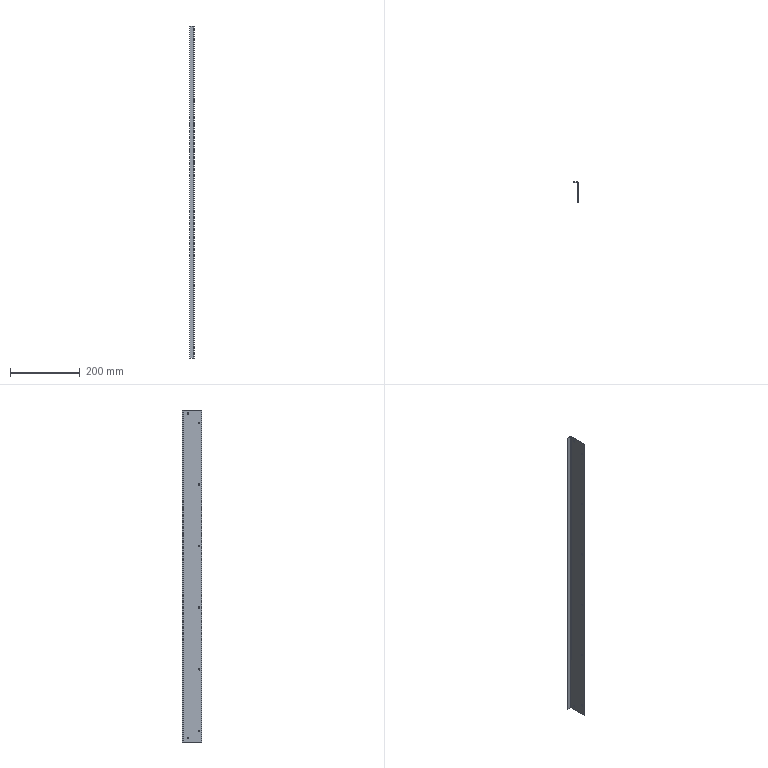Part | STEP file | 866-BDO024-95-07A_default | 1 solid | 26 faces | box 13.5 x 56.5 x 954 mm | volume 96451 mm3 | cylinder 18 | plane 8 | commonest cylinder face diameters 4.5 x16 3 x1 6 x1
STEP:
#1=CARTESIAN_POINT('',(1.5,40.,9.25));
#2=VERTEX_POINT('',#1);
#3=CARTESIAN_POINT('',(1.5,40.,13.75));
#4=VERTEX_POINT('',#3);
#5=CARTESIAN_POINT('',(1.5,40.,11.5));
#6=DIRECTION('',(-1.,0.,0.));
#7=DIRECTION('',(0.,0.,1.));
#8=AXIS2_PLACEMENT_3D('',#5,#6,#7);
#9=CIRCLE('',#8,2.25);
#10=EDGE_CURVE('',#2,#4,#9,.T.);
#11=ORIENTED_EDGE('',*,*,#10,.F.);
#12=CARTESIAN_POINT('',(0.,40.,9.25));
#13=VERTEX_POINT('',#12);
#14=CARTESIAN_POINT('',(0.,40.,9.25));
#15=DIRECTION('',(-1.,0.,0.));
#16=VECTOR('',#15,1000.);
#17=LINE('',#14,#16);
#18=EDGE_CURVE('',#2,#13,#17,.T.);
#19=ORIENTED_EDGE('',*,*,#18,.T.);
#20=CARTESIAN_POINT('',(0.,40.,13.75));
#21=VERTEX_POINT('',#20);
#22=CARTESIAN_POINT('',(0.,40.,11.5));
#23=DIRECTION('',(1.,0.,0.));
#24=DIRECTION('',(0.,0.,1.));
#25=AXIS2_PLACEMENT_3D('',#22,#23,#24);
#26=CIRCLE('',#25,2.25);
#27=EDGE_CURVE('',#21,#13,#26,.T.);
#28=ORIENTED_EDGE('',*,*,#27,.F.);
#29=CARTESIAN_POINT('',(0.,40.,13.75));
#30=DIRECTION('',(-1.,0.,0.));
#31=VECTOR('',#30,1000.);
#32=LINE('',#29,#31);
#33=EDGE_CURVE('',#4,#21,#32,.T.);
#34=ORIENTED_EDGE('',*,*,#33,.F.);
#35=EDGE_LOOP('',(#11,#19,#28,#34));
#36=FACE_OUTER_BOUND('',#35,.T.);
#37=CARTESIAN_POINT('',(0.,40.,11.5));
#38=DIRECTION('',(-1.,0.,0.));
#39=DIRECTION('',(0.,0.,1.));
#40=AXIS2_PLACEMENT_3D('',#37,#38,#39);
#41=CYLINDRICAL_SURFACE('',#40,2.25);
#42=ADVANCED_FACE('',(#36),#41,.F.);
#43=CARTESIAN_POINT('',(1.5,40.,941.75));
#44=VERTEX_POINT('',#43);
#45=CARTESIAN_POINT('',(1.5,40.,946.25));
#46=VERTEX_POINT('',#45);
#47=CARTESIAN_POINT('',(1.5,40.,944.));
#48=DIRECTION('',(-1.,0.,0.));
#49=DIRECTION('',(0.,0.,1.));
#50=AXIS2_PLACEMENT_3D('',#47,#48,#49);
#51=CIRCLE('',#50,2.25);
#52=EDGE_CURVE('',#44,#46,#51,.T.);
#53=ORIENTED_EDGE('',*,*,#52,.F.);
#54=CARTESIAN_POINT('',(0.,40.,941.75));
#55=VERTEX_POINT('',#54);
#56=CARTESIAN_POINT('',(0.,40.,941.75));
#57=DIRECTION('',(-1.,0.,0.));
#58=VECTOR('',#57,1000.);
#59=LINE('',#56,#58);
#60=EDGE_CURVE('',#44,#55,#59,.T.);
#61=ORIENTED_EDGE('',*,*,#60,.T.);
#62=CARTESIAN_POINT('',(0.,40.,946.25));
#63=VERTEX_POINT('',#62);
#64=CARTESIAN_POINT('',(0.,40.,944.));
#65=DIRECTION('',(1.,0.,0.));
#66=DIRECTION('',(0.,0.,1.));
#67=AXIS2_PLACEMENT_3D('',#64,#65,#66);
#68=CIRCLE('',#67,2.25);
#69=EDGE_CURVE('',#63,#55,#68,.T.);
#70=ORIENTED_EDGE('',*,*,#69,.F.);
#71=CARTESIAN_POINT('',(0.,40.,946.25));
#72=DIRECTION('',(-1.,0.,0.));
#73=VECTOR('',#72,1000.);
#74=LINE('',#71,#73);
#75=EDGE_CURVE('',#46,#63,#74,.T.);
#76=ORIENTED_EDGE('',*,*,#75,.F.);
#77=EDGE_LOOP('',(#53,#61,#70,#76));
#78=FACE_OUTER_BOUND('',#77,.T.);
#79=CARTESIAN_POINT('',(0.,40.,944.));
#80=DIRECTION('',(-1.,0.,0.));
#81=DIRECTION('',(0.,0.,1.));
#82=AXIS2_PLACEMENT_3D('',#79,#80,#81);
#83=CYLINDRICAL_SURFACE('',#82,2.25);
#84=ADVANCED_FACE('',(#78),#83,.F.);
#85=CARTESIAN_POINT('',(1.5,7.5,914.75));
#86=VERTEX_POINT('',#85);
#87=CARTESIAN_POINT('',(1.5,7.5,919.25));
#88=VERTEX_POINT('',#87);
#89=CARTESIAN_POINT('',(1.5,7.5,917.));
#90=DIRECTION('',(-1.,0.,0.));
#91=DIRECTION('',(0.,0.,1.));
#92=AXIS2_PLACEMENT_3D('',#89,#90,#91);
#93=CIRCLE('',#92,2.25);
#94=EDGE_CURVE('',#86,#88,#93,.T.);
#95=ORIENTED_EDGE('',*,*,#94,.F.);
#96=CARTESIAN_POINT('',(0.,7.5,914.75));
#97=VERTEX_POINT('',#96);
#98=CARTESIAN_POINT('',(0.,7.5,914.75));
#99=DIRECTION('',(-1.,0.,0.));
#100=VECTOR('',#99,1000.);
#101=LINE('',#98,#100);
#102=EDGE_CURVE('',#86,#97,#101,.T.);
#103=ORIENTED_EDGE('',*,*,#102,.T.);
#104=CARTESIAN_POINT('',(0.,7.5,919.25));
#105=VERTEX_POINT('',#104);
#106=CARTESIAN_POINT('',(0.,7.5,917.));
#107=DIRECTION('',(1.,0.,0.));
#108=DIRECTION('',(0.,0.,1.));
#109=AXIS2_PLACEMENT_3D('',#106,#107,#108);
#110=CIRCLE('',#109,2.25);
#111=EDGE_CURVE('',#105,#97,#110,.T.);
#112=ORIENTED_EDGE('',*,*,#111,.F.);
#113=CARTESIAN_POINT('',(0.,7.5,919.25));
#114=DIRECTION('',(-1.,0.,0.));
#115=VECTOR('',#114,1000.);
#116=LINE('',#113,#115);
#117=EDGE_CURVE('',#88,#105,#116,.T.);
#118=ORIENTED_EDGE('',*,*,#117,.F.);
#119=EDGE_LOOP('',(#95,#103,#112,#118));
#120=FACE_OUTER_BOUND('',#119,.T.);
#121=CARTESIAN_POINT('',(0.,7.5,917.));
#122=DIRECTION('',(-1.,0.,0.));
#123=DIRECTION('',(0.,0.,1.));
#124=AXIS2_PLACEMENT_3D('',#121,#122,#123);
#125=CYLINDRICAL_SURFACE('',#124,2.25);
#126=ADVANCED_FACE('',(#120),#125,.F.);
#127=CARTESIAN_POINT('',(1.5,7.5,737.75));
#128=VERTEX_POINT('',#127);
#129=CARTESIAN_POINT('',(1.5,7.5,742.25));
#130=VERTEX_POINT('',#129);
#131=CARTESIAN_POINT('',(1.5,7.5,740.));
#132=DIRECTION('',(-1.,0.,0.));
#133=DIRECTION('',(0.,0.,1.));
#134=AXIS2_PLACEMENT_3D('',#131,#132,#133);
#135=CIRCLE('',#134,2.25);
#136=EDGE_CURVE('',#128,#130,#135,.T.);
#137=ORIENTED_EDGE('',*,*,#136,.F.);
#138=CARTESIAN_POINT('',(0.,7.5,737.75));
#139=VERTEX_POINT('',#138);
#140=CARTESIAN_POINT('',(0.,7.5,737.75));
#141=DIRECTION('',(-1.,0.,0.));
#142=VECTOR('',#141,1000.);
#143=LINE('',#140,#142);
#144=EDGE_CURVE('',#128,#139,#143,.T.);
#145=ORIENTED_EDGE('',*,*,#144,.T.);
#146=CARTESIAN_POINT('',(0.,7.5,742.25));
#147=VERTEX_POINT('',#146);
#148=CARTESIAN_POINT('',(0.,7.5,740.));
#149=DIRECTION('',(1.,0.,0.));
#150=DIRECTION('',(0.,0.,1.));
#151=AXIS2_PLACEMENT_3D('',#148,#149,#150);
#152=CIRCLE('',#151,2.25);
#153=EDGE_CURVE('',#147,#139,#152,.T.);
#154=ORIENTED_EDGE('',*,*,#153,.F.);
#155=CARTESIAN_POINT('',(0.,7.5,742.25));
#156=DIRECTION('',(-1.,0.,0.));
#157=VECTOR('',#156,1000.);
#158=LINE('',#155,#157);
#159=EDGE_CURVE('',#130,#147,#158,.T.);
#160=ORIENTED_EDGE('',*,*,#159,.F.);
#161=EDGE_LOOP('',(#137,#145,#154,#160));
#162=FACE_OUTER_BOUND('',#161,.T.);
#163=CARTESIAN_POINT('',(0.,7.5,740.));
#164=DIRECTION('',(-1.,0.,0.));
#165=DIRECTION('',(0.,0.,1.));
#166=AXIS2_PLACEMENT_3D('',#163,#164,#165);
#167=CYLINDRICAL_SURFACE('',#166,2.25);
#168=ADVANCED_FACE('',(#162),#167,.F.);
#169=CARTESIAN_POINT('',(1.5,7.5,560.75));
#170=VERTEX_POINT('',#169);
#171=CARTESIAN_POINT('',(1.5,7.5,565.25));
#172=VERTEX_POINT('',#171);
#173=CARTESIAN_POINT('',(1.5,7.5,563.));
#174=DIRECTION('',(-1.,0.,0.));
#175=DIRECTION('',(0.,0.,1.));
#176=AXIS2_PLACEMENT_3D('',#173,#174,#175);
#177=CIRCLE('',#176,2.25);
#178=EDGE_CURVE('',#170,#172,#177,.T.);
#179=ORIENTED_EDGE('',*,*,#178,.F.);
#180=CARTESIAN_POINT('',(0.,7.5,560.75));
#181=VERTEX_POINT('',#180);
#182=CARTESIAN_POINT('',(0.,7.5,560.75));
#183=DIRECTION('',(-1.,0.,0.));
#184=VECTOR('',#183,1000.);
#185=LINE('',#182,#184);
#186=EDGE_CURVE('',#170,#181,#185,.T.);
#187=ORIENTED_EDGE('',*,*,#186,.T.);
#188=CARTESIAN_POINT('',(0.,7.5,565.25));
#189=VERTEX_POINT('',#188);
#190=CARTESIAN_POINT('',(0.,7.5,563.));
#191=DIRECTION('',(1.,0.,0.));
#192=DIRECTION('',(0.,0.,1.));
#193=AXIS2_PLACEMENT_3D('',#190,#191,#192);
#194=CIRCLE('',#193,2.25);
#195=EDGE_CURVE('',#189,#181,#194,.T.);
#196=ORIENTED_EDGE('',*,*,#195,.F.);
#197=CARTESIAN_POINT('',(0.,7.5,565.25));
#198=DIRECTION('',(-1.,0.,0.));
#199=VECTOR('',#198,1000.);
#200=LINE('',#197,#199);
#201=EDGE_CURVE('',#172,#189,#200,.T.);
#202=ORIENTED_EDGE('',*,*,#201,.F.);
#203=EDGE_LOOP('',(#179,#187,#196,#202));
#204=FACE_OUTER_BOUND('',#203,.T.);
#205=CARTESIAN_POINT('',(0.,7.5,563.));
#206=DIRECTION('',(-1.,0.,0.));
#207=DIRECTION('',(0.,0.,1.));
#208=AXIS2_PLACEMENT_3D('',#205,#206,#207);
#209=CYLINDRICAL_SURFACE('',#208,2.25);
#210=ADVANCED_FACE('',(#204),#209,.F.);
#211=CARTESIAN_POINT('',(1.5,7.5,383.75));
#212=VERTEX_POINT('',#211);
#213=CARTESIAN_POINT('',(1.5,7.5,388.25));
#214=VERTEX_POINT('',#213);
#215=CARTESIAN_POINT('',(1.5,7.5,386.));
#216=DIRECTION('',(-1.,0.,0.));
#217=DIRECTION('',(0.,0.,1.));
#218=AXIS2_PLACEMENT_3D('',#215,#216,#217);
#219=CIRCLE('',#218,2.25);
#220=EDGE_CURVE('',#212,#214,#219,.T.);
#221=ORIENTED_EDGE('',*,*,#220,.F.);
#222=CARTESIAN_POINT('',(0.,7.5,383.75));
#223=VERTEX_POINT('',#222);
#224=CARTESIAN_POINT('',(0.,7.5,383.75));
#225=DIRECTION('',(-1.,0.,0.));
#226=VECTOR('',#225,1000.);
#227=LINE('',#224,#226);
#228=EDGE_CURVE('',#212,#223,#227,.T.);
#229=ORIENTED_EDGE('',*,*,#228,.T.);
#230=CARTESIAN_POINT('',(0.,7.5,388.25));
#231=VERTEX_POINT('',#230);
#232=CARTESIAN_POINT('',(0.,7.5,386.));
#233=DIRECTION('',(1.,0.,0.));
#234=DIRECTION('',(0.,0.,1.));
#235=AXIS2_PLACEMENT_3D('',#232,#233,#234);
#236=CIRCLE('',#235,2.25);
#237=EDGE_CURVE('',#231,#223,#236,.T.);
#238=ORIENTED_EDGE('',*,*,#237,.F.);
#239=CARTESIAN_POINT('',(0.,7.5,388.25));
#240=DIRECTION('',(-1.,0.,0.));
#241=VECTOR('',#240,1000.);
#242=LINE('',#239,#241);
#243=EDGE_CURVE('',#214,#231,#242,.T.);
#244=ORIENTED_EDGE('',*,*,#243,.F.);
#245=EDGE_LOOP('',(#221,#229,#238,#244));
#246=FACE_OUTER_BOUND('',#245,.T.);
#247=CARTESIAN_POINT('',(0.,7.5,386.));
#248=DIRECTION('',(-1.,0.,0.));
#249=DIRECTION('',(0.,0.,1.));
#250=AXIS2_PLACEMENT_3D('',#247,#248,#249);
#251=CYLINDRICAL_SURFACE('',#250,2.25);
#252=ADVANCED_FACE('',(#246),#251,.F.);
#253=CARTESIAN_POINT('',(1.5,7.5,206.75));
#254=VERTEX_POINT('',#253);
#255=CARTESIAN_POINT('',(1.5,7.5,211.25));
#256=VERTEX_POINT('',#255);
#257=CARTESIAN_POINT('',(1.5,7.5,209.));
#258=DIRECTION('',(-1.,0.,0.));
#259=DIRECTION('',(0.,0.,1.));
#260=AXIS2_PLACEMENT_3D('',#257,#258,#259);
#261=CIRCLE('',#260,2.25);
#262=EDGE_CURVE('',#254,#256,#261,.T.);
#263=ORIENTED_EDGE('',*,*,#262,.F.);
#264=CARTESIAN_POINT('',(0.,7.5,206.75));
#265=VERTEX_POINT('',#264);
#266=CARTESIAN_POINT('',(0.,7.5,206.75));
#267=DIRECTION('',(-1.,0.,0.));
#268=VECTOR('',#267,1000.);
#269=LINE('',#266,#268);
#270=EDGE_CURVE('',#254,#265,#269,.T.);
#271=ORIENTED_EDGE('',*,*,#270,.T.);
#272=CARTESIAN_POINT('',(0.,7.5,211.25));
#273=VERTEX_POINT('',#272);
#274=CARTESIAN_POINT('',(0.,7.5,209.));
#275=DIRECTION('',(1.,0.,0.));
#276=DIRECTION('',(0.,0.,1.));
#277=AXIS2_PLACEMENT_3D('',#274,#275,#276);
#278=CIRCLE('',#277,2.25);
#279=EDGE_CURVE('',#273,#265,#278,.T.);
#280=ORIENTED_EDGE('',*,*,#279,.F.);
#281=CARTESIAN_POINT('',(0.,7.5,211.25));
#282=DIRECTION('',(-1.,0.,0.));
#283=VECTOR('',#282,1000.);
#284=LINE('',#281,#283);
#285=EDGE_CURVE('',#256,#273,#284,.T.);
#286=ORIENTED_EDGE('',*,*,#285,.F.);
#287=EDGE_LOOP('',(#263,#271,#280,#286));
#288=FACE_OUTER_BOUND('',#287,.T.);
#289=CARTESIAN_POINT('',(0.,7.5,209.));
#290=DIRECTION('',(-1.,0.,0.));
#291=DIRECTION('',(0.,0.,1.));
#292=AXIS2_PLACEMENT_3D('',#289,#290,#291);
#293=CYLINDRICAL_SURFACE('',#292,2.25);
#294=ADVANCED_FACE('',(#288),#293,.F.);
#295=CARTESIAN_POINT('',(1.5,7.5,29.75));
#296=VERTEX_POINT('',#295);
#297=CARTESIAN_POINT('',(1.5,7.5,34.25));
#298=VERTEX_POINT('',#297);
#299=CARTESIAN_POINT('',(1.5,7.5,32.));
#300=DIRECTION('',(-1.,0.,0.));
#301=DIRECTION('',(0.,0.,1.));
#302=AXIS2_PLACEMENT_3D('',#299,#300,#301);
#303=CIRCLE('',#302,2.25);
#304=EDGE_CURVE('',#296,#298,#303,.T.);
#305=ORIENTED_EDGE('',*,*,#304,.F.);
#306=CARTESIAN_POINT('',(0.,7.5,29.75));
#307=VERTEX_POINT('',#306);
#308=CARTESIAN_POINT('',(0.,7.5,29.75));
#309=DIRECTION('',(-1.,0.,0.));
#310=VECTOR('',#309,1000.);
#311=LINE('',#308,#310);
#312=EDGE_CURVE('',#296,#307,#311,.T.);
#313=ORIENTED_EDGE('',*,*,#312,.T.);
#314=CARTESIAN_POINT('',(0.,7.5,34.25));
#315=VERTEX_POINT('',#314);
#316=CARTESIAN_POINT('',(0.,7.5,32.));
#317=DIRECTION('',(1.,0.,0.));
#318=DIRECTION('',(0.,0.,1.));
#319=AXIS2_PLACEMENT_3D('',#316,#317,#318);
#320=CIRCLE('',#319,2.25);
#321=EDGE_CURVE('',#315,#307,#320,.T.);
#322=ORIENTED_EDGE('',*,*,#321,.F.);
#323=CARTESIAN_POINT('',(0.,7.5,34.25));
#324=DIRECTION('',(-1.,0.,0.));
#325=VECTOR('',#324,1000.);
#326=LINE('',#323,#325);
#327=EDGE_CURVE('',#298,#315,#326,.T.);
#328=ORIENTED_EDGE('',*,*,#327,.F.);
#329=EDGE_LOOP('',(#305,#313,#322,#328));
#330=FACE_OUTER_BOUND('',#329,.T.);
#331=CARTESIAN_POINT('',(0.,7.5,32.));
#332=DIRECTION('',(-1.,0.,0.));
#333=DIRECTION('',(0.,0.,1.));
#334=AXIS2_PLACEMENT_3D('',#331,#332,#333);
#335=CYLINDRICAL_SURFACE('',#334,2.25);
#336=ADVANCED_FACE('',(#330),#335,.F.);
#337=CARTESIAN_POINT('',(0.,0.,954.));
#338=VERTEX_POINT('',#337);
#339=CARTESIAN_POINT('',(0.,53.5,954.));
#340=VERTEX_POINT('',#339);
#341=CARTESIAN_POINT('',(0.,0.,954.));
#342=DIRECTION('',(0.,1.,0.));
#343=VECTOR('',#342,1000.);
#344=LINE('',#341,#343);
#345=EDGE_CURVE('',#338,#340,#344,.T.);
#346=ORIENTED_EDGE('',*,*,#345,.T.);
#347=CARTESIAN_POINT('',(0.,53.5,0.));
#348=VERTEX_POINT('',#347);
#349=CARTESIAN_POINT('',(0.,53.5,954.));
#350=DIRECTION('',(0.,0.,-1.));
#351=VECTOR('',#350,1000.);
#352=LINE('',#349,#351);
#353=EDGE_CURVE('',#340,#348,#352,.T.);
#354=ORIENTED_EDGE('',*,*,#353,.T.);
#355=CARTESIAN_POINT('',(0.,0.,0.));
#356=VERTEX_POINT('',#355);
#357=CARTESIAN_POINT('',(0.,0.,0.));
#358=DIRECTION('',(0.,-1.,0.));
#359=VECTOR('',#358,1000.);
#360=LINE('',#357,#359);
#361=EDGE_CURVE('',#348,#356,#360,.T.);
#362=ORIENTED_EDGE('',*,*,#361,.T.);
#363=CARTESIAN_POINT('',(0.,0.,954.));
#364=DIRECTION('',(0.,0.,1.));
#365=VECTOR('',#364,1000.);
#366=LINE('',#363,#365);
#367=EDGE_CURVE('',#356,#338,#366,.T.);
#368=ORIENTED_EDGE('',*,*,#367,.T.);
#369=EDGE_LOOP('',(#346,#354,#362,#368));
#370=FACE_OUTER_BOUND('',#369,.T.);
#371=ORIENTED_EDGE('',*,*,#27,.T.);
#372=CARTESIAN_POINT('',(0.,40.,11.5));
#373=DIRECTION('',(1.,0.,0.));
#374=DIRECTION('',(0.,0.,1.));
#375=AXIS2_PLACEMENT_3D('',#372,#373,#374);
#376=CIRCLE('',#375,2.25);
#377=EDGE_CURVE('',#13,#21,#376,.T.);
#378=ORIENTED_EDGE('',*,*,#377,.T.);
#379=EDGE_LOOP('',(#371,#378));
#380=FACE_BOUND('',#379,.T.);
#381=ORIENTED_EDGE('',*,*,#69,.T.);
#382=CARTESIAN_POINT('',(0.,40.,944.));
#383=DIRECTION('',(1.,0.,0.));
#384=DIRECTION('',(0.,0.,1.));
#385=AXIS2_PLACEMENT_3D('',#382,#383,#384);
#386=CIRCLE('',#385,2.25);
#387=EDGE_CURVE('',#55,#63,#386,.T.);
#388=ORIENTED_EDGE('',*,*,#387,.T.);
#389=EDGE_LOOP('',(#381,#388));
#390=FACE_BOUND('',#389,.T.);
#391=ORIENTED_EDGE('',*,*,#111,.T.);
#392=CARTESIAN_POINT('',(0.,7.5,917.));
#393=DIRECTION('',(1.,0.,0.));
#394=DIRECTION('',(0.,0.,1.));
#395=AXIS2_PLACEMENT_3D('',#392,#393,#394);
#396=CIRCLE('',#395,2.25);
#397=EDGE_CURVE('',#97,#105,#396,.T.);
#398=ORIENTED_EDGE('',*,*,#397,.T.);
#399=EDGE_LOOP('',(#391,#398));
#400=FACE_BOUND('',#399,.T.);
#401=ORIENTED_EDGE('',*,*,#153,.T.);
#402=CARTESIAN_POINT('',(0.,7.5,740.));
#403=DIRECTION('',(1.,0.,0.));
#404=DIRECTION('',(0.,0.,1.));
#405=AXIS2_PLACEMENT_3D('',#402,#403,#404);
#406=CIRCLE('',#405,2.25);
#407=EDGE_CURVE('',#139,#147,#406,.T.);
#408=ORIENTED_EDGE('',*,*,#407,.T.);
#409=EDGE_LOOP('',(#401,#408));
#410=FACE_BOUND('',#409,.T.);
#411=ORIENTED_EDGE('',*,*,#195,.T.);
#412=CARTESIAN_POINT('',(0.,7.5,563.));
#413=DIRECTION('',(1.,0.,0.));
#414=DIRECTION('',(0.,0.,1.));
#415=AXIS2_PLACEMENT_3D('',#412,#413,#414);
#416=CIRCLE('',#415,2.25);
#417=EDGE_CURVE('',#181,#189,#416,.T.);
#418=ORIENTED_EDGE('',*,*,#417,.T.);
#419=EDGE_LOOP('',(#411,#418));
#420=FACE_BOUND('',#419,.T.);
#421=ORIENTED_EDGE('',*,*,#237,.T.);
#422=CARTESIAN_POINT('',(0.,7.5,386.));
#423=DIRECTION('',(1.,0.,0.));
#424=DIRECTION('',(0.,0.,1.));
#425=AXIS2_PLACEMENT_3D('',#422,#423,#424);
#426=CIRCLE('',#425,2.25);
#427=EDGE_CURVE('',#223,#231,#426,.T.);
#428=ORIENTED_EDGE('',*,*,#427,.T.);
#429=EDGE_LOOP('',(#421,#428));
#430=FACE_BOUND('',#429,.T.);
#431=ORIENTED_EDGE('',*,*,#279,.T.);
#432=CARTESIAN_POINT('',(0.,7.5,209.));
#433=DIRECTION('',(1.,0.,0.));
#434=DIRECTION('',(0.,0.,1.));
#435=AXIS2_PLACEMENT_3D('',#432,#433,#434);
#436=CIRCLE('',#435,2.25);
#437=EDGE_CURVE('',#265,#273,#436,.T.);
#438=ORIENTED_EDGE('',*,*,#437,.T.);
#439=EDGE_LOOP('',(#431,#438));
#440=FACE_BOUND('',#439,.T.);
#441=ORIENTED_EDGE('',*,*,#321,.T.);
#442=CARTESIAN_POINT('',(0.,7.5,32.));
#443=DIRECTION('',(1.,0.,0.));
#444=DIRECTION('',(0.,0.,1.));
#445=AXIS2_PLACEMENT_3D('',#442,#443,#444);
#446=CIRCLE('',#445,2.25);
#447=EDGE_CURVE('',#307,#315,#446,.T.);
#448=ORIENTED_EDGE('',*,*,#447,.T.);
#449=EDGE_LOOP('',(#441,#448));
#450=FACE_BOUND('',#449,.T.);
#451=CARTESIAN_POINT('',(0.,0.,954.));
#452=DIRECTION('',(-1.,0.,0.));
#453=DIRECTION('',(0.,0.,1.));
#454=AXIS2_PLACEMENT_3D('',#451,#452,#453);
#455=PLANE('',#454);
#456=ADVANCED_FACE('',(#370,#380,#390,#400,#410,#420,#430,#440,#450),#455,.T.);
#457=ORIENTED_EDGE('',*,*,#353,.F.);
#458=CARTESIAN_POINT('',(-1.5,55.,954.));
#459=VERTEX_POINT('',#458);
#460=CARTESIAN_POINT('',(-1.5,53.5,954.));
#461=DIRECTION('',(0.,0.,-1.));
#462=DIRECTION('',(-1.,0.,0.));
#463=AXIS2_PLACEMENT_3D('',#460,#461,#462);
#464=CIRCLE('',#463,1.5);
#465=EDGE_CURVE('',#459,#340,#464,.T.);
#466=ORIENTED_EDGE('',*,*,#465,.F.);
#467=CARTESIAN_POINT('',(-1.5,55.,0.));
#468=VERTEX_POINT('',#467);
#469=CARTESIAN_POINT('',(-1.5,55.,954.));
#470=DIRECTION('',(0.,0.,1.));
#471=VECTOR('',#470,1000.);
#472=LINE('',#469,#471);
#473=EDGE_CURVE('',#468,#459,#472,.T.);
#474=ORIENTED_EDGE('',*,*,#473,.F.);
#475=CARTESIAN_POINT('',(-1.5,53.5,0.));
#476=DIRECTION('',(0.,0.,1.));
#477=DIRECTION('',(-1.,0.,0.));
#478=AXIS2_PLACEMENT_3D('',#475,#476,#477);
#479=CIRCLE('',#478,1.5);
#480=EDGE_CURVE('',#348,#468,#479,.T.);
#481=ORIENTED_EDGE('',*,*,#480,.F.);
#482=EDGE_LOOP('',(#457,#466,#474,#481));
#483=FACE_OUTER_BOUND('',#482,.T.);
#484=CARTESIAN_POINT('',(-1.5,53.5,954.));
#485=DIRECTION('',(0.,0.,-1.));
#486=DIRECTION('',(-1.,0.,0.));
#487=AXIS2_PLACEMENT_3D('',#484,#485,#486);
#488=CYLINDRICAL_SURFACE('',#487,1.5);
#489=ADVANCED_FACE('',(#483),#488,.F.);
#490=CARTESIAN_POINT('',(1.5,53.5,954.));
#491=VERTEX_POINT('',#490);
#492=CARTESIAN_POINT('',(1.5,0.,954.));
#493=VERTEX_POINT('',#492);
#494=CARTESIAN_POINT('',(1.5,53.5,954.));
#495=DIRECTION('',(0.,-1.,0.));
#496=VECTOR('',#495,1000.);
#497=LINE('',#494,#496);
#498=EDGE_CURVE('',#491,#493,#497,.T.);
#499=ORIENTED_EDGE('',*,*,#498,.F.);
#500=CARTESIAN_POINT('',(-1.5,56.5,954.));
#501=VERTEX_POINT('',#500);
#502=CARTESIAN_POINT('',(-1.5,53.5,954.));
#503=DIRECTION('',(0.,0.,1.));
#504=DIRECTION('',(-1.,0.,0.));
#505=AXIS2_PLACEMENT_3D('',#502,#503,#504);
#506=CIRCLE('',#505,3.);
#507=EDGE_CURVE('',#491,#501,#506,.T.);
#508=ORIENTED_EDGE('',*,*,#507,.T.);
#509=CARTESIAN_POINT('',(-12.,56.5,954.));
#510=VERTEX_POINT('',#509);
#511=CARTESIAN_POINT('',(1.5,56.5,954.));
#512=DIRECTION('',(-1.,0.,0.));
#513=VECTOR('',#512,1000.);
#514=LINE('',#511,#513);
#515=EDGE_CURVE('',#501,#510,#514,.T.);
#516=ORIENTED_EDGE('',*,*,#515,.T.);
#517=CARTESIAN_POINT('',(-12.,55.,954.));
#518=VERTEX_POINT('',#517);
#519=CARTESIAN_POINT('',(-12.,55.,954.));
#520=DIRECTION('',(0.,1.,0.));
#521=VECTOR('',#520,1000.);
#522=LINE('',#519,#521);
#523=EDGE_CURVE('',#518,#510,#522,.T.);
#524=ORIENTED_EDGE('',*,*,#523,.F.);
#525=CARTESIAN_POINT('',(0.,55.,954.));
#526=DIRECTION('',(-1.,0.,0.));
#527=VECTOR('',#526,1000.);
#528=LINE('',#525,#527);
#529=EDGE_CURVE('',#459,#518,#528,.T.);
#530=ORIENTED_EDGE('',*,*,#529,.F.);
#531=ORIENTED_EDGE('',*,*,#465,.T.);
#532=ORIENTED_EDGE('',*,*,#345,.F.);
#533=CARTESIAN_POINT('',(-1.5,0.,954.));
#534=DIRECTION('',(-1.,0.,0.));
#535=VECTOR('',#534,1000.);
#536=LINE('',#533,#535);
#537=EDGE_CURVE('',#493,#338,#536,.T.);
#538=ORIENTED_EDGE('',*,*,#537,.F.);
#539=EDGE_LOOP('',(#499,#508,#516,#524,#530,#531,#532,#538));
#540=FACE_OUTER_BOUND('',#539,.T.);
#541=CARTESIAN_POINT('',(-1.5,53.5,954.));
#542=DIRECTION('',(0.,0.,-1.));
#543=DIRECTION('',(-1.,0.,0.));
#544=AXIS2_PLACEMENT_3D('',#541,#542,#543);
#545=PLANE('',#544);
#546=ADVANCED_FACE('',(#540),#545,.F.);
#547=ORIENTED_EDGE('',*,*,#537,.T.);
#548=ORIENTED_EDGE('',*,*,#367,.F.);
#549=CARTESIAN_POINT('',(1.5,0.,0.));
#550=VERTEX_POINT('',#549);
#551=CARTESIAN_POINT('',(1.5,0.,0.));
#552=DIRECTION('',(1.,0.,0.));
#553=VECTOR('',#552,1000.);
#554=LINE('',#551,#553);
#555=EDGE_CURVE('',#356,#550,#554,.T.);
#556=ORIENTED_EDGE('',*,*,#555,.T.);
#557=CARTESIAN_POINT('',(1.5,0.,954.));
#558=DIRECTION('',(0.,0.,1.));
#559=VECTOR('',#558,1000.);
#560=LINE('',#557,#559);
#561=EDGE_CURVE('',#550,#493,#560,.T.);
#562=ORIENTED_EDGE('',*,*,#561,.T.);
#563=EDGE_LOOP('',(#547,#548,#556,#562));
#564=FACE_OUTER_BOUND('',#563,.T.);
#565=CARTESIAN_POINT('',(1.5,0.,954.));
#566=DIRECTION('',(0.,-1.,0.));
#567=DIRECTION('',(0.,0.,-1.));
#568=AXIS2_PLACEMENT_3D('',#565,#566,#567);
#569=PLANE('',#568);
#570=ADVANCED_FACE('',(#564),#569,.T.);
#571=CARTESIAN_POINT('',(1.5,53.5,0.));
#572=VERTEX_POINT('',#571);
#573=CARTESIAN_POINT('',(1.5,56.5,0.));
#574=DIRECTION('',(0.,-1.,0.));
#575=VECTOR('',#574,1000.);
#576=LINE('',#573,#575);
#577=EDGE_CURVE('',#572,#550,#576,.T.);
#578=ORIENTED_EDGE('',*,*,#577,.T.);
#579=ORIENTED_EDGE('',*,*,#555,.F.);
#580=ORIENTED_EDGE('',*,*,#361,.F.);
#581=ORIENTED_EDGE('',*,*,#480,.T.);
#582=CARTESIAN_POINT('',(-12.,55.,0.));
#583=VERTEX_POINT('',#582);
#584=CARTESIAN_POINT('',(0.,55.,0.));
#585=DIRECTION('',(1.,0.,0.));
#586=VECTOR('',#585,1000.);
#587=LINE('',#584,#586);
#588=EDGE_CURVE('',#583,#468,#587,.T.);
#589=ORIENTED_EDGE('',*,*,#588,.F.);
#590=CARTESIAN_POINT('',(-12.,56.5,0.));
#591=VERTEX_POINT('',#590);
#592=CARTESIAN_POINT('',(-12.,55.,0.));
#593=DIRECTION('',(0.,-1.,0.));
#594=VECTOR('',#593,1000.);
#595=LINE('',#592,#594);
#596=EDGE_CURVE('',#591,#583,#595,.T.);
#597=ORIENTED_EDGE('',*,*,#596,.F.);
#598=CARTESIAN_POINT('',(-1.5,56.5,0.));
#599=VERTEX_POINT('',#598);
#600=CARTESIAN_POINT('',(-1.5,56.5,0.));
#601=DIRECTION('',(1.,0.,0.));
#602=VECTOR('',#601,1000.);
#603=LINE('',#600,#602);
#604=EDGE_CURVE('',#591,#599,#603,.T.);
#605=ORIENTED_EDGE('',*,*,#604,.T.);
#606=CARTESIAN_POINT('',(-1.5,53.5,0.));
#607=DIRECTION('',(0.,0.,-1.));
#608=DIRECTION('',(-1.,0.,0.));
#609=AXIS2_PLACEMENT_3D('',#606,#607,#608);
#610=CIRCLE('',#609,3.);
#611=EDGE_CURVE('',#599,#572,#610,.T.);
#612=ORIENTED_EDGE('',*,*,#611,.T.);
#613=EDGE_LOOP('',(#578,#579,#580,#581,#589,#597,#605,#612));
#614=FACE_OUTER_BOUND('',#613,.T.);
#615=CARTESIAN_POINT('',(-1.5,56.5,0.));
#616=DIRECTION('',(0.,0.,-1.));
#617=DIRECTION('',(-1.,0.,0.));
#618=AXIS2_PLACEMENT_3D('',#615,#616,#617);
#619=PLANE('',#618);
#620=ADVANCED_FACE('',(#614),#619,.T.);
#621=ORIENTED_EDGE('',*,*,#18,.F.);
#622=CARTESIAN_POINT('',(1.5,40.,11.5));
#623=DIRECTION('',(-1.,0.,0.));
#624=DIRECTION('',(0.,0.,1.));
#625=AXIS2_PLACEMENT_3D('',#622,#623,#624);
#626=CIRCLE('',#625,2.25);
#627=EDGE_CURVE('',#4,#2,#626,.T.);
#628=ORIENTED_EDGE('',*,*,#627,.F.);
#629=ORIENTED_EDGE('',*,*,#33,.T.);
#630=ORIENTED_EDGE('',*,*,#377,.F.);
#631=EDGE_LOOP('',(#621,#628,#629,#630));
#632=FACE_OUTER_BOUND('',#631,.T.);
#633=CARTESIAN_POINT('',(0.,40.,11.5));
#634=DIRECTION('',(-1.,0.,0.));
#635=DIRECTION('',(0.,0.,1.));
#636=AXIS2_PLACEMENT_3D('',#633,#634,#635);
#637=CYLINDRICAL_SURFACE('',#636,2.25);
#638=ADVANCED_FACE('',(#632),#637,.F.);
#639=ORIENTED_EDGE('',*,*,#60,.F.);
#640=CARTESIAN_POINT('',(1.5,40.,944.));
#641=DIRECTION('',(-1.,0.,0.));
#642=DIRECTION('',(0.,0.,1.));
#643=AXIS2_PLACEMENT_3D('',#640,#641,#642);
#644=CIRCLE('',#643,2.25);
#645=EDGE_CURVE('',#46,#44,#644,.T.);
#646=ORIENTED_EDGE('',*,*,#645,.F.);
#647=ORIENTED_EDGE('',*,*,#75,.T.);
#648=ORIENTED_EDGE('',*,*,#387,.F.);
#649=EDGE_LOOP('',(#639,#646,#647,#648));
#650=FACE_OUTER_BOUND('',#649,.T.);
#651=CARTESIAN_POINT('',(0.,40.,944.));
#652=DIRECTION('',(-1.,0.,0.));
#653=DIRECTION('',(0.,0.,1.));
#654=AXIS2_PLACEMENT_3D('',#651,#652,#653);
#655=CYLINDRICAL_SURFACE('',#654,2.25);
#656=ADVANCED_FACE('',(#650),#655,.F.);
#657=ORIENTED_EDGE('',*,*,#102,.F.);
#658=CARTESIAN_POINT('',(1.5,7.5,917.));
#659=DIRECTION('',(-1.,0.,0.));
#660=DIRECTION('',(0.,0.,1.));
#661=AXIS2_PLACEMENT_3D('',#658,#659,#660);
#662=CIRCLE('',#661,2.25);
#663=EDGE_CURVE('',#88,#86,#662,.T.);
#664=ORIENTED_EDGE('',*,*,#663,.F.);
#665=ORIENTED_EDGE('',*,*,#117,.T.);
#666=ORIENTED_EDGE('',*,*,#397,.F.);
#667=EDGE_LOOP('',(#657,#664,#665,#666));
#668=FACE_OUTER_BOUND('',#667,.T.);
#669=CARTESIAN_POINT('',(0.,7.5,917.));
#670=DIRECTION('',(-1.,0.,0.));
#671=DIRECTION('',(0.,0.,1.));
#672=AXIS2_PLACEMENT_3D('',#669,#670,#671);
#673=CYLINDRICAL_SURFACE('',#672,2.25);
#674=ADVANCED_FACE('',(#668),#673,.F.);
#675=ORIENTED_EDGE('',*,*,#144,.F.);
#676=CARTESIAN_POINT('',(1.5,7.5,740.));
#677=DIRECTION('',(-1.,0.,0.));
#678=DIRECTION('',(0.,0.,1.));
#679=AXIS2_PLACEMENT_3D('',#676,#677,#678);
#680=CIRCLE('',#679,2.25);
#681=EDGE_CURVE('',#130,#128,#680,.T.);
#682=ORIENTED_EDGE('',*,*,#681,.F.);
#683=ORIENTED_EDGE('',*,*,#159,.T.);
#684=ORIENTED_EDGE('',*,*,#407,.F.);
#685=EDGE_LOOP('',(#675,#682,#683,#684));
#686=FACE_OUTER_BOUND('',#685,.T.);
#687=CARTESIAN_POINT('',(0.,7.5,740.));
#688=DIRECTION('',(-1.,0.,0.));
#689=DIRECTION('',(0.,0.,1.));
#690=AXIS2_PLACEMENT_3D('',#687,#688,#689);
#691=CYLINDRICAL_SURFACE('',#690,2.25);
#692=ADVANCED_FACE('',(#686),#691,.F.);
#693=ORIENTED_EDGE('',*,*,#186,.F.);
#694=CARTESIAN_POINT('',(1.5,7.5,563.));
#695=DIRECTION('',(-1.,0.,0.));
#696=DIRECTION('',(0.,0.,1.));
#697=AXIS2_PLACEMENT_3D('',#694,#695,#696);
#698=CIRCLE('',#697,2.25);
#699=EDGE_CURVE('',#172,#170,#698,.T.);
#700=ORIENTED_EDGE('',*,*,#699,.F.);
#701=ORIENTED_EDGE('',*,*,#201,.T.);
#702=ORIENTED_EDGE('',*,*,#417,.F.);
#703=EDGE_LOOP('',(#693,#700,#701,#702));
#704=FACE_OUTER_BOUND('',#703,.T.);
#705=CARTESIAN_POINT('',(0.,7.5,563.));
#706=DIRECTION('',(-1.,0.,0.));
#707=DIRECTION('',(0.,0.,1.));
#708=AXIS2_PLACEMENT_3D('',#705,#706,#707);
#709=CYLINDRICAL_SURFACE('',#708,2.25);
#710=ADVANCED_FACE('',(#704),#709,.F.);
#711=ORIENTED_EDGE('',*,*,#228,.F.);
#712=CARTESIAN_POINT('',(1.5,7.5,386.));
#713=DIRECTION('',(-1.,0.,0.));
#714=DIRECTION('',(0.,0.,1.));
#715=AXIS2_PLACEMENT_3D('',#712,#713,#714);
#716=CIRCLE('',#715,2.25);
#717=EDGE_CURVE('',#214,#212,#716,.T.);
#718=ORIENTED_EDGE('',*,*,#717,.F.);
#719=ORIENTED_EDGE('',*,*,#243,.T.);
#720=ORIENTED_EDGE('',*,*,#427,.F.);
#721=EDGE_LOOP('',(#711,#718,#719,#720));
#722=FACE_OUTER_BOUND('',#721,.T.);
#723=CARTESIAN_POINT('',(0.,7.5,386.));
#724=DIRECTION('',(-1.,0.,0.));
#725=DIRECTION('',(0.,0.,1.));
#726=AXIS2_PLACEMENT_3D('',#723,#724,#725);
#727=CYLINDRICAL_SURFACE('',#726,2.25);
#728=ADVANCED_FACE('',(#722),#727,.F.);
#729=ORIENTED_EDGE('',*,*,#270,.F.);
#730=CARTESIAN_POINT('',(1.5,7.5,209.));
#731=DIRECTION('',(-1.,0.,0.));
#732=DIRECTION('',(0.,0.,1.));
#733=AXIS2_PLACEMENT_3D('',#730,#731,#732);
#734=CIRCLE('',#733,2.25);
#735=EDGE_CURVE('',#256,#254,#734,.T.);
#736=ORIENTED_EDGE('',*,*,#735,.F.);
#737=ORIENTED_EDGE('',*,*,#285,.T.);
#738=ORIENTED_EDGE('',*,*,#437,.F.);
#739=EDGE_LOOP('',(#729,#736,#737,#738));
#740=FACE_OUTER_BOUND('',#739,.T.);
#741=CARTESIAN_POINT('',(0.,7.5,209.));
#742=DIRECTION('',(-1.,0.,0.));
#743=DIRECTION('',(0.,0.,1.));
#744=AXIS2_PLACEMENT_3D('',#741,#742,#743);
#745=CYLINDRICAL_SURFACE('',#744,2.25);
#746=ADVANCED_FACE('',(#740),#745,.F.);
#747=ORIENTED_EDGE('',*,*,#312,.F.);
#748=CARTESIAN_POINT('',(1.5,7.5,32.));
#749=DIRECTION('',(-1.,0.,0.));
#750=DIRECTION('',(0.,0.,1.));
#751=AXIS2_PLACEMENT_3D('',#748,#749,#750);
#752=CIRCLE('',#751,2.25);
#753=EDGE_CURVE('',#298,#296,#752,.T.);
#754=ORIENTED_EDGE('',*,*,#753,.F.);
#755=ORIENTED_EDGE('',*,*,#327,.T.);
#756=ORIENTED_EDGE('',*,*,#447,.F.);
#757=EDGE_LOOP('',(#747,#754,#755,#756));
#758=FACE_OUTER_BOUND('',#757,.T.);
#759=CARTESIAN_POINT('',(0.,7.5,32.));
#760=DIRECTION('',(-1.,0.,0.));
#761=DIRECTION('',(0.,0.,1.));
#762=AXIS2_PLACEMENT_3D('',#759,#760,#761);
#763=CYLINDRICAL_SURFACE('',#762,2.25);
#764=ADVANCED_FACE('',(#758),#763,.F.);
#765=ORIENTED_EDGE('',*,*,#529,.T.);
#766=CARTESIAN_POINT('',(-12.,55.,954.));
#767=DIRECTION('',(0.,0.,-1.));
#768=VECTOR('',#767,1000.);
#769=LINE('',#766,#768);
#770=EDGE_CURVE('',#518,#583,#769,.T.);
#771=ORIENTED_EDGE('',*,*,#770,.T.);
#772=ORIENTED_EDGE('',*,*,#588,.T.);
#773=ORIENTED_EDGE('',*,*,#473,.T.);
#774=EDGE_LOOP('',(#765,#771,#772,#773));
#775=FACE_OUTER_BOUND('',#774,.T.);
#776=CARTESIAN_POINT('',(0.,55.,954.));
#777=DIRECTION('',(0.,-1.,0.));
#778=DIRECTION('',(0.,0.,-1.));
#779=AXIS2_PLACEMENT_3D('',#776,#777,#778);
#780=PLANE('',#779);
#781=ADVANCED_FACE('',(#775),#780,.T.);
#782=CARTESIAN_POINT('',(1.5,53.5,954.));
#783=DIRECTION('',(0.,0.,-1.));
#784=VECTOR('',#783,1000.);
#785=LINE('',#782,#784);
#786=EDGE_CURVE('',#491,#572,#785,.T.);
#787=ORIENTED_EDGE('',*,*,#786,.F.);
#788=ORIENTED_EDGE('',*,*,#498,.T.);
#789=ORIENTED_EDGE('',*,*,#561,.F.);
#790=ORIENTED_EDGE('',*,*,#577,.F.);
#791=EDGE_LOOP('',(#787,#788,#789,#790));
#792=FACE_OUTER_BOUND('',#791,.T.);
#793=ORIENTED_EDGE('',*,*,#627,.T.);
#794=ORIENTED_EDGE('',*,*,#10,.T.);
#795=EDGE_LOOP('',(#793,#794));
#796=FACE_BOUND('',#795,.T.);
#797=ORIENTED_EDGE('',*,*,#645,.T.);
#798=ORIENTED_EDGE('',*,*,#52,.T.);
#799=EDGE_LOOP('',(#797,#798));
#800=FACE_BOUND('',#799,.T.);
#801=ORIENTED_EDGE('',*,*,#663,.T.);
#802=ORIENTED_EDGE('',*,*,#94,.T.);
#803=EDGE_LOOP('',(#801,#802));
#804=FACE_BOUND('',#803,.T.);
#805=ORIENTED_EDGE('',*,*,#681,.T.);
#806=ORIENTED_EDGE('',*,*,#136,.T.);
#807=EDGE_LOOP('',(#805,#806));
#808=FACE_BOUND('',#807,.T.);
#809=ORIENTED_EDGE('',*,*,#699,.T.);
#810=ORIENTED_EDGE('',*,*,#178,.T.);
#811=EDGE_LOOP('',(#809,#810));
#812=FACE_BOUND('',#811,.T.);
#813=ORIENTED_EDGE('',*,*,#717,.T.);
#814=ORIENTED_EDGE('',*,*,#220,.T.);
#815=EDGE_LOOP('',(#813,#814));
#816=FACE_BOUND('',#815,.T.);
#817=ORIENTED_EDGE('',*,*,#735,.T.);
#818=ORIENTED_EDGE('',*,*,#262,.T.);
#819=EDGE_LOOP('',(#817,#818));
#820=FACE_BOUND('',#819,.T.);
#821=ORIENTED_EDGE('',*,*,#753,.T.);
#822=ORIENTED_EDGE('',*,*,#304,.T.);
#823=EDGE_LOOP('',(#821,#822));
#824=FACE_BOUND('',#823,.T.);
#825=CARTESIAN_POINT('',(1.5,0.,954.));
#826=DIRECTION('',(-1.,0.,0.));
#827=DIRECTION('',(0.,0.,1.));
#828=AXIS2_PLACEMENT_3D('',#825,#826,#827);
#829=PLANE('',#828);
#830=ADVANCED_FACE('',(#792,#796,#800,#804,#808,#812,#816,#820,#824),#829,.F.);
#831=ORIENTED_EDGE('',*,*,#507,.F.);
#832=ORIENTED_EDGE('',*,*,#786,.T.);
#833=ORIENTED_EDGE('',*,*,#611,.F.);
#834=CARTESIAN_POINT('',(-1.5,56.5,954.));
#835=DIRECTION('',(0.,0.,1.));
#836=VECTOR('',#835,1000.);
#837=LINE('',#834,#836);
#838=EDGE_CURVE('',#599,#501,#837,.T.);
#839=ORIENTED_EDGE('',*,*,#838,.T.);
#840=EDGE_LOOP('',(#831,#832,#833,#839));
#841=FACE_OUTER_BOUND('',#840,.T.);
#842=CARTESIAN_POINT('',(-1.5,53.5,954.));
#843=DIRECTION('',(0.,0.,-1.));
#844=DIRECTION('',(-1.,0.,0.));
#845=AXIS2_PLACEMENT_3D('',#842,#843,#844);
#846=CYLINDRICAL_SURFACE('',#845,3.);
#847=ADVANCED_FACE('',(#841),#846,.T.);
#848=ORIENTED_EDGE('',*,*,#523,.T.);
#849=CARTESIAN_POINT('',(-12.,56.5,954.));
#850=DIRECTION('',(0.,0.,-1.));
#851=VECTOR('',#850,1000.);
#852=LINE('',#849,#851);
#853=EDGE_CURVE('',#510,#591,#852,.T.);
#854=ORIENTED_EDGE('',*,*,#853,.T.);
#855=ORIENTED_EDGE('',*,*,#596,.T.);
#856=ORIENTED_EDGE('',*,*,#770,.F.);
#857=EDGE_LOOP('',(#848,#854,#855,#856));
#858=FACE_OUTER_BOUND('',#857,.T.);
#859=CARTESIAN_POINT('',(-12.,55.,954.));
#860=DIRECTION('',(-1.,0.,0.));
#861=DIRECTION('',(0.,0.,1.));
#862=AXIS2_PLACEMENT_3D('',#859,#860,#861);
#863=PLANE('',#862);
#864=ADVANCED_FACE('',(#858),#863,.T.);
#865=ORIENTED_EDGE('',*,*,#853,.F.);
#866=ORIENTED_EDGE('',*,*,#515,.F.);
#867=ORIENTED_EDGE('',*,*,#838,.F.);
#868=ORIENTED_EDGE('',*,*,#604,.F.);
#869=EDGE_LOOP('',(#865,#866,#867,#868));
#870=FACE_OUTER_BOUND('',#869,.T.);
#871=CARTESIAN_POINT('',(0.,56.5,954.));
#872=DIRECTION('',(0.,-1.,0.));
#873=DIRECTION('',(0.,0.,-1.));
#874=AXIS2_PLACEMENT_3D('',#871,#872,#873);
#875=PLANE('',#874);
#876=ADVANCED_FACE('',(#870),#875,.F.);
#877=CLOSED_SHELL('',(#42,#84,#126,#168,#210,#252,#294,#336,#456,#489,#546,#570,#620,#638,#656,#674,#692,#710,#728,#746,#764,#781,#830,#847,#864,#876));
#878=MANIFOLD_SOLID_BREP('',#877);
#879=CARTESIAN_POINT('',(0.,0.,0.));
#880=DIRECTION('',(0.,0.,1.));
#881=DIRECTION('',(1.,0.,0.));
#882=AXIS2_PLACEMENT_3D('',#879,#880,#881);
#883=(LENGTH_UNIT()NAMED_UNIT(*)SI_UNIT(.MILLI.,.METRE.));
#884=UNCERTAINTY_MEASURE_WITH_UNIT(LENGTH_MEASURE(0.00001),#883,'','');
#885=(NAMED_UNIT(*)PLANE_ANGLE_UNIT()SI_UNIT($,.RADIAN.));
#886=(NAMED_UNIT(*)SI_UNIT($,.STERADIAN.)SOLID_ANGLE_UNIT());
#887=(GEOMETRIC_REPRESENTATION_CONTEXT(3)GLOBAL_UNCERTAINTY_ASSIGNED_CONTEXT((#884))GLOBAL_UNIT_ASSIGNED_CONTEXT((#883,#885,#886))REPRESENTATION_CONTEXT('',''));
#888=ADVANCED_BREP_SHAPE_REPRESENTATION('',(#878,#882),#887);